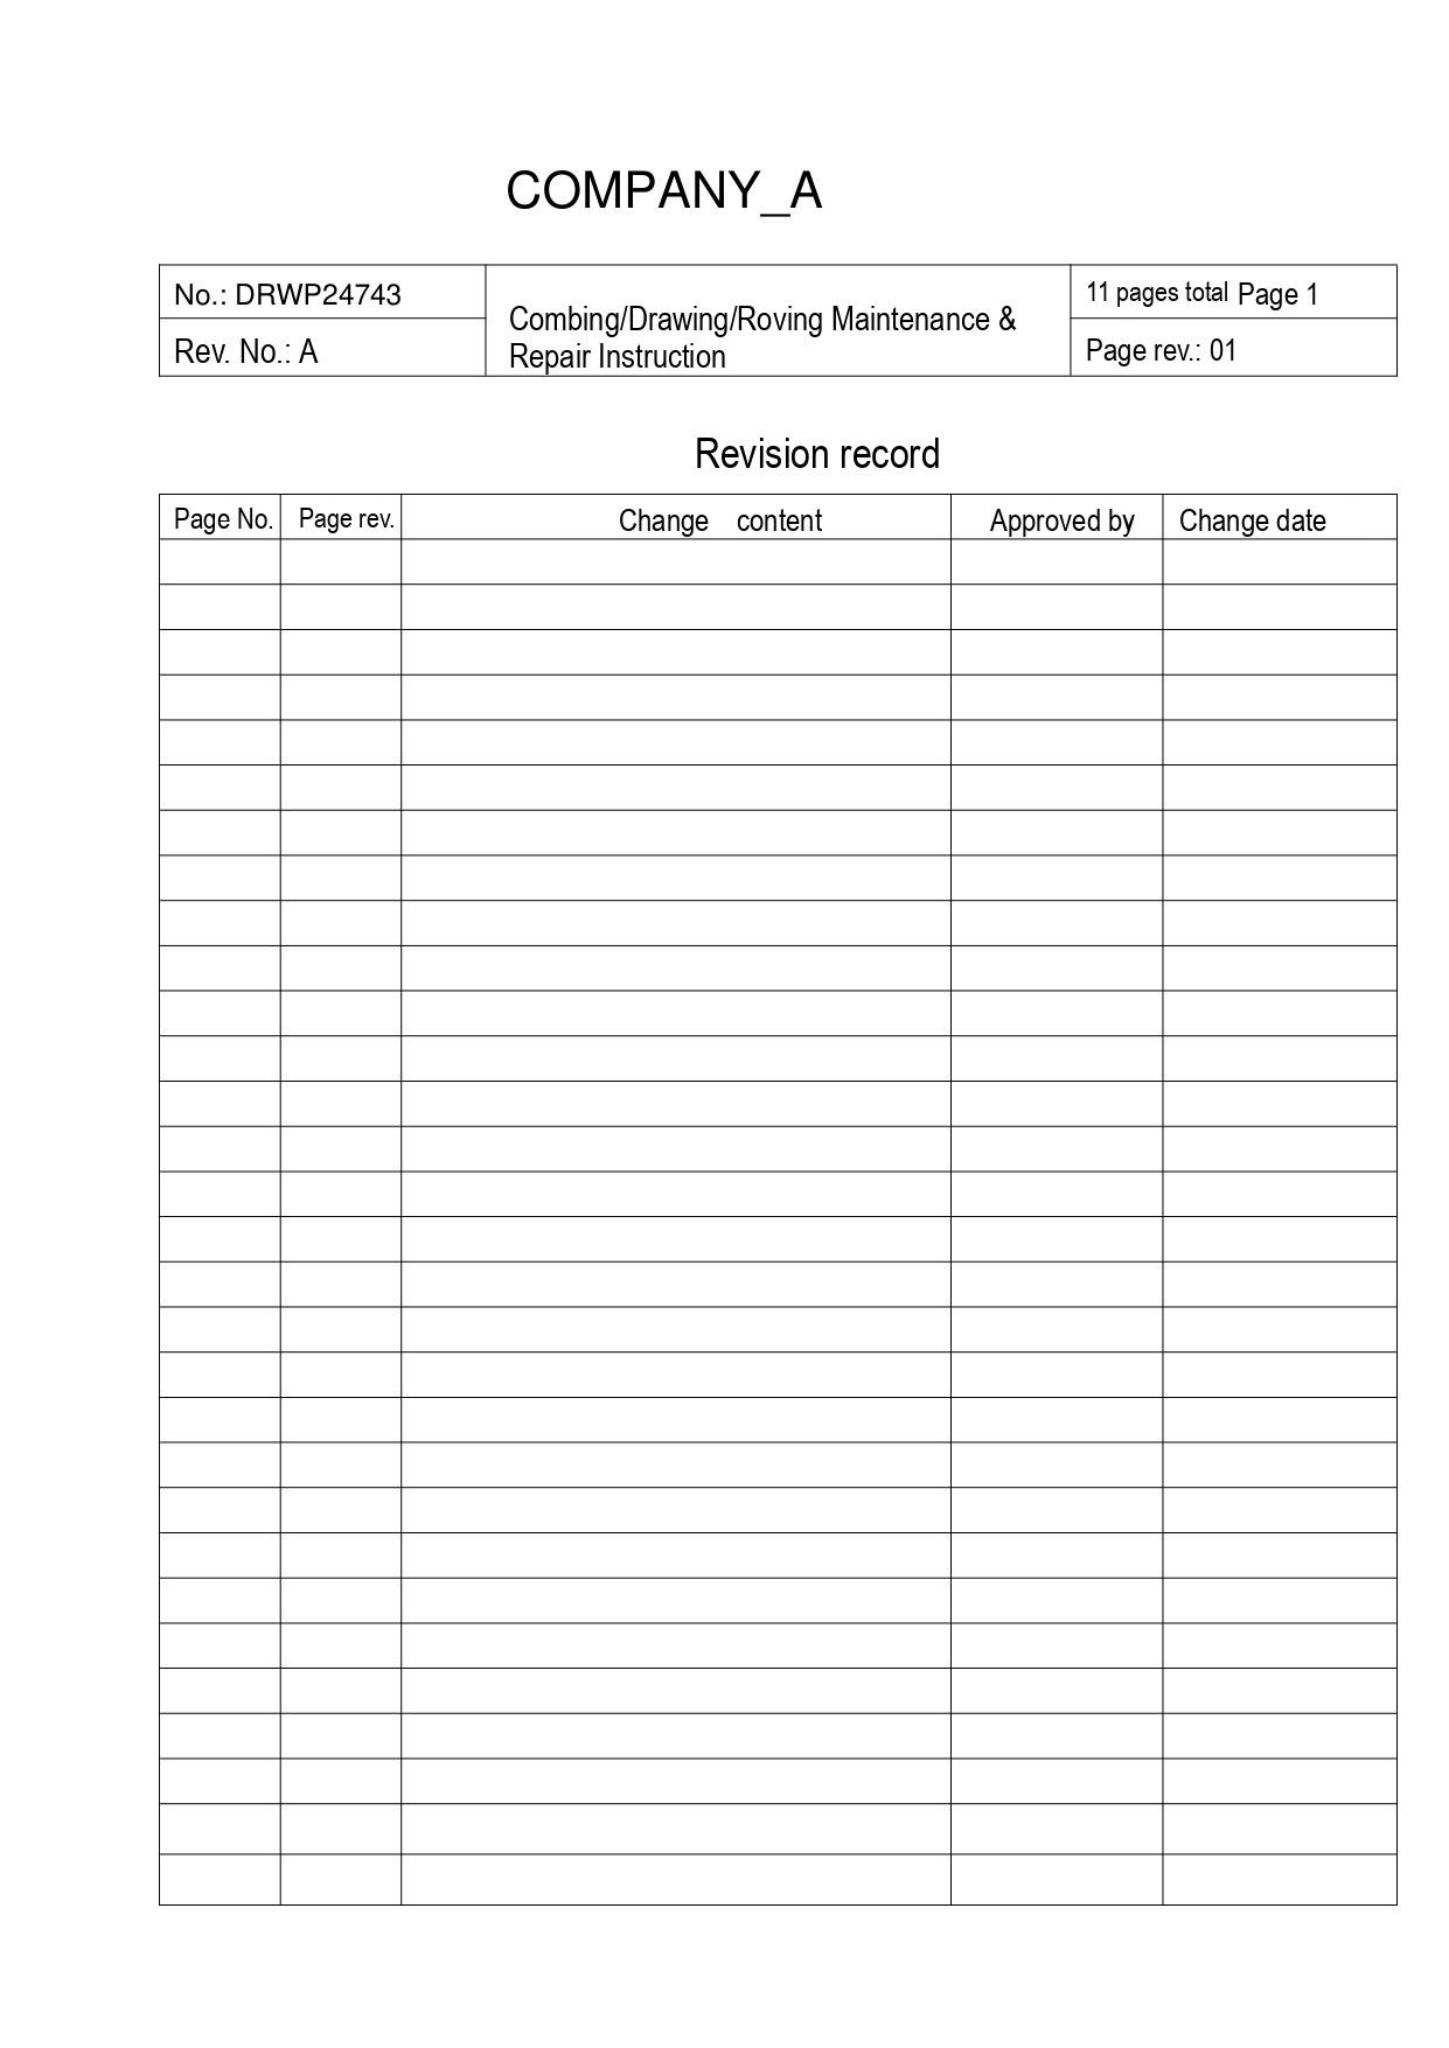COMPANY_A

| No.: DRWP24743 | Combing/Drawing/Roving Maintenance & Repair Instruction | 11 pages total Page 1 |
|---|---|---|
| Rev. No.: A | | Page rev.: 01 |

Revision record

| Page No. | Page rev. | Change content | Approved by | Change date |
|---|---|---|---|---|
| | | | | |
| | | | | |
| | | | | |
| | | | | |
| | | | | |
| | | | | |
| | | | | |
| | | | | |
| | | | | |
| | | | | |
| | | | | |
| | | | | |
| | | | | |
| | | | | |
| | | | | |
| | | | | |
| | | | | |
| | | | | |
| | | | | |
| | | | | |
| | | | | |
| | | | | |
| | | | | |
| | | | | |
| | | | | |
| | | | | |
| | | | | |
| | | | | |
| | | | | |
| | | | | |
| | | | | |
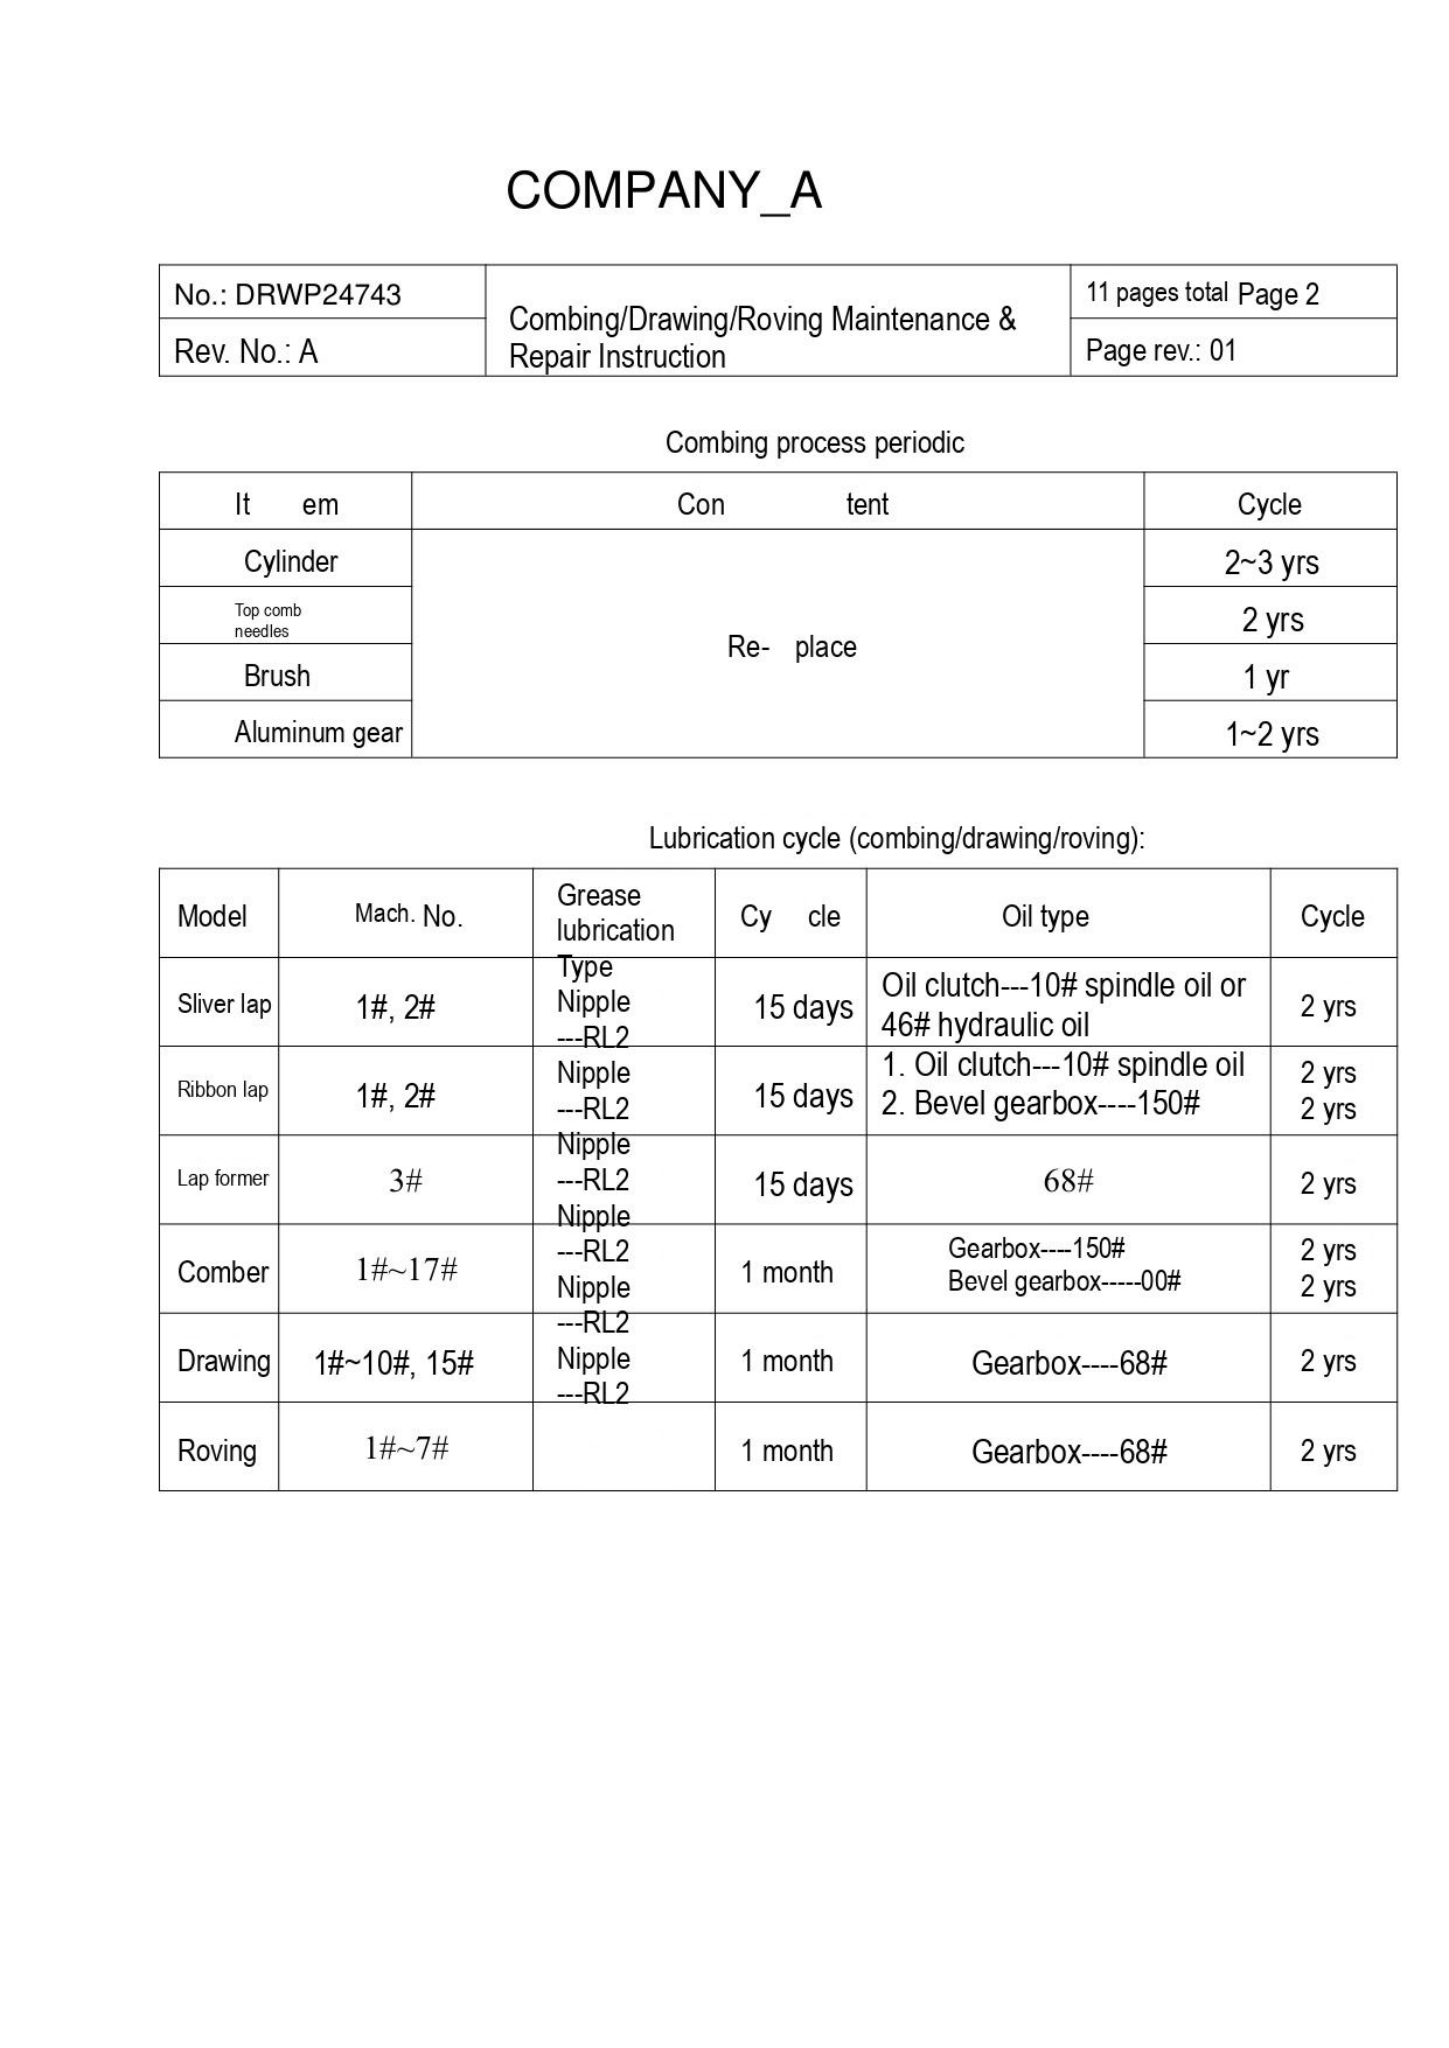COMPANY_A

| No.: DRWP24743 | Combing/Drawing/Roving Maintenance & Repair Instruction | 11 pages total Page 2 |
|---|---|---|
| Rev. No.: A | | Page rev.: 01 |

Combing process periodic

| It em | Con tent | Cycle |
|---|---|---|
| Cylinder | Re- place | 2~3 yrs |
| Top comb needles | | 2 yrs |
| Brush | | 1 yr |
| Aluminum gear | | 1~2 yrs |

Lubrication cycle (combing/drawing/roving):

| Model | Mach. No. | Grease lubrication Type | Cy cle | Oil type | Cycle |
|---|---|---|---|---|---|
| Sliver lap | 1#, 2# | Nipple ---RL2 | 15 days | Oil clutch---10# spindle oil or 46# hydraulic oil | 2 yrs |
| Ribbon lap | 1#, 2# | Nipple ---RL2 | 15 days | 1. Oil clutch---10# spindle oil<br>2. Bevel gearbox----150# | 2 yrs<br>2 yrs |
| Lap former | 3# | Nipple ---RL2 | 15 days | 68# | 2 yrs |
| Comber | 1#~17# | Nipple ---RL2<br>Nipple ---RL2 | 1 month | Gearbox----150#<br>Bevel gearbox-----00# | 2 yrs<br>2 yrs |
| Drawing | 1#~10#, 15# | Nipple ---RL2 | 1 month | Gearbox----68# | 2 yrs |
| Roving | 1#~7# | | 1 month | Gearbox----68# | 2 yrs |
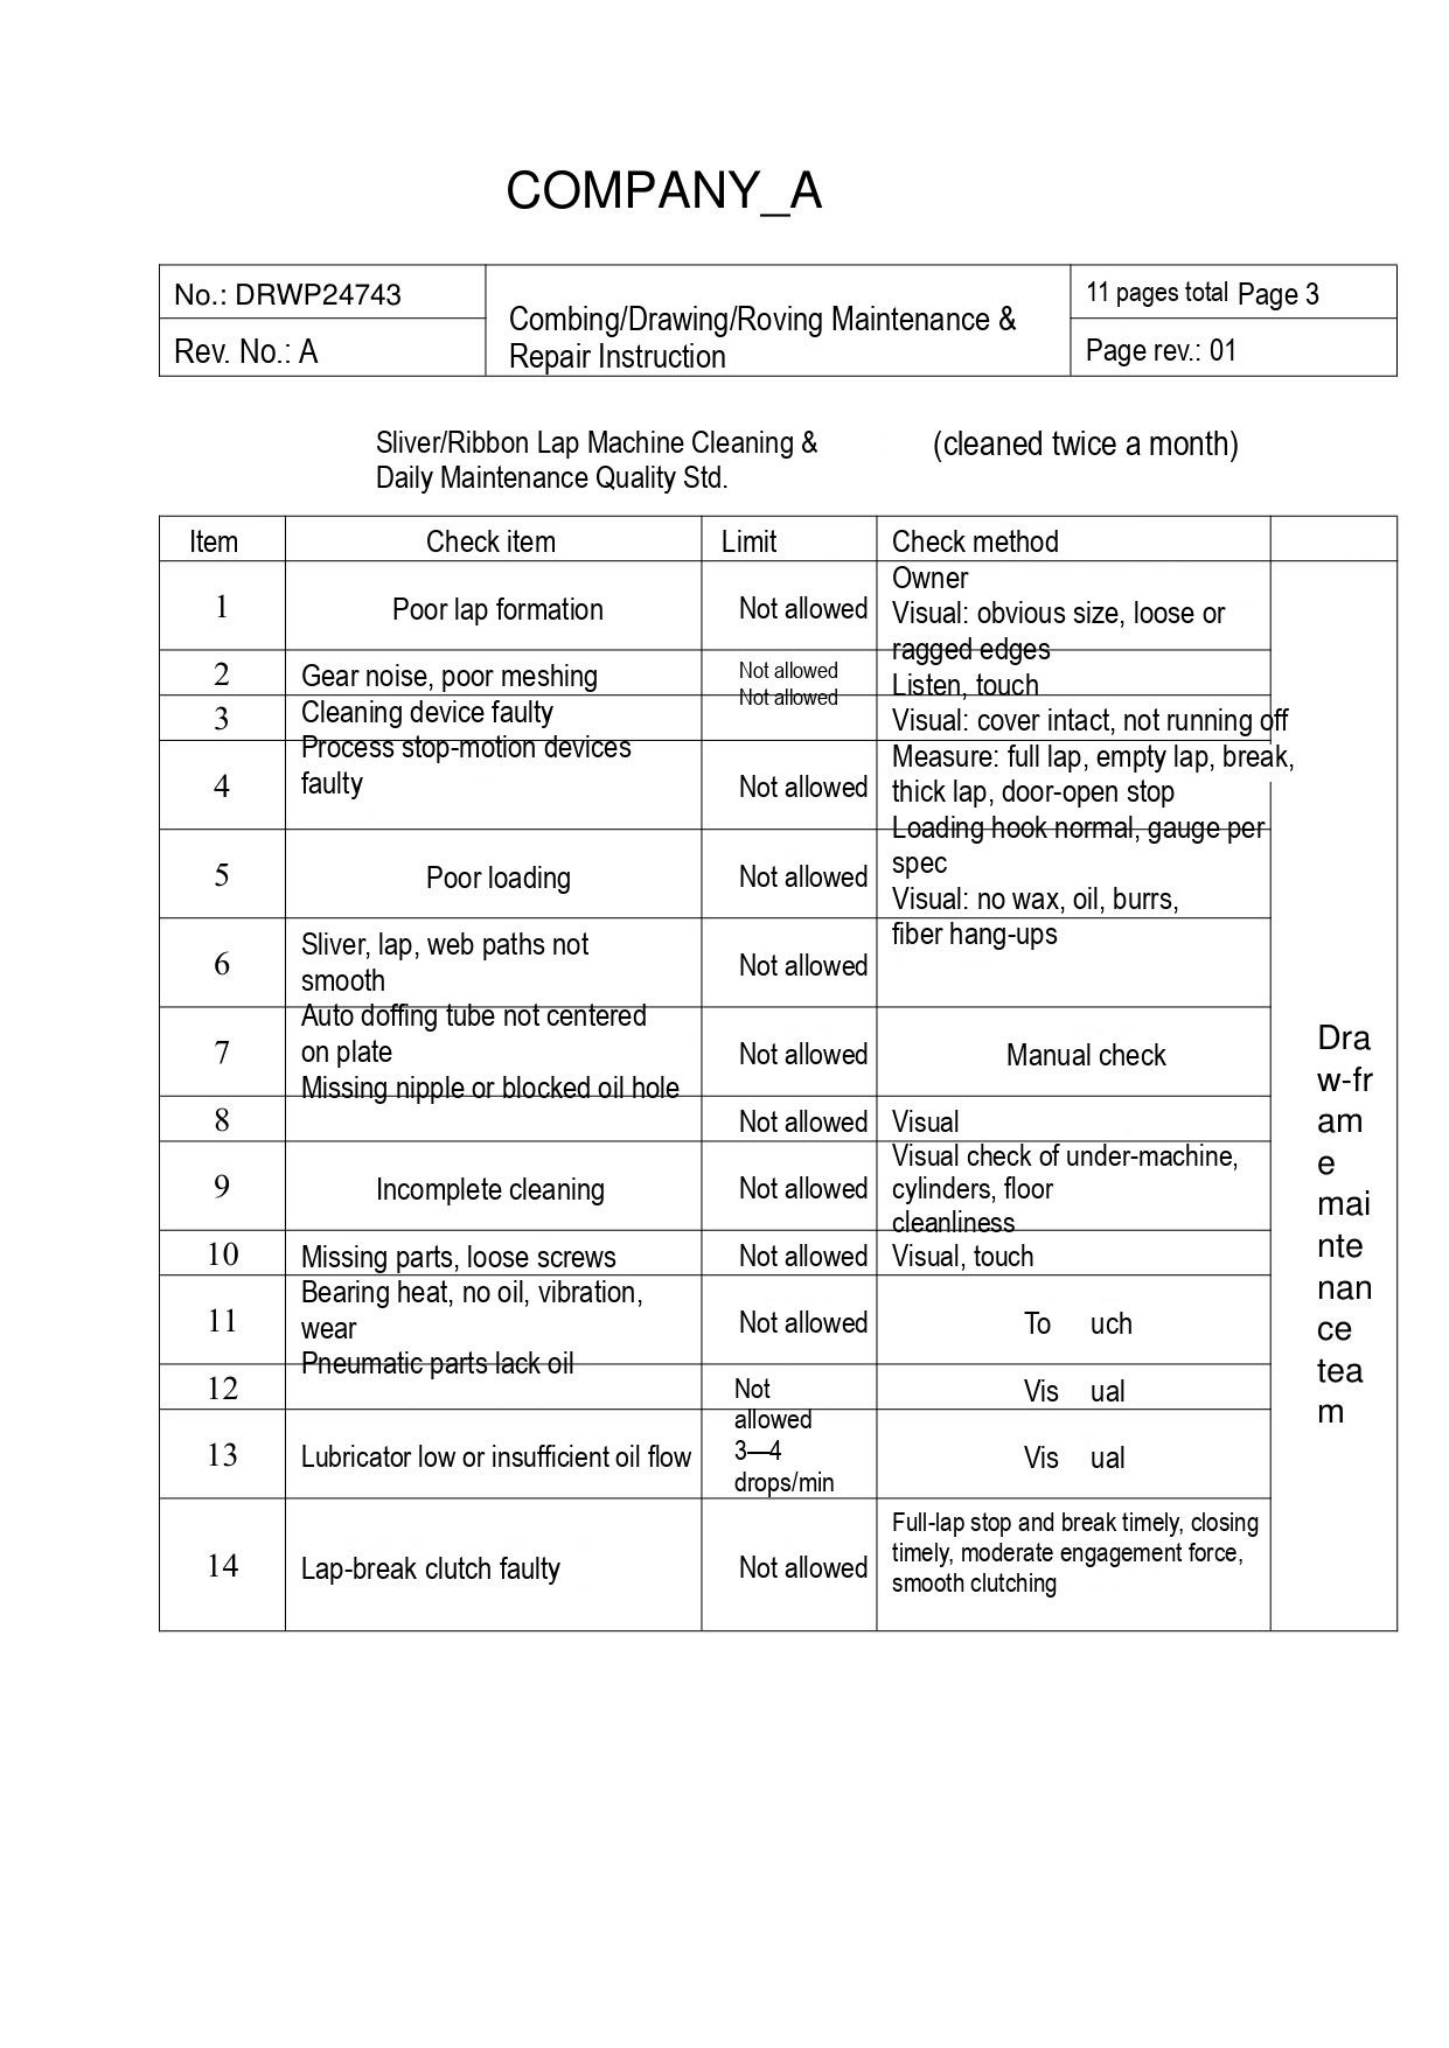# COMPANY_A

| No.: DRWP24743 | Combing/Drawing/Roving Maintenance & Repair Instruction | 11 pages total Page 3 |
|---|---|---|
| Rev. No.: A | | Page rev.: 01 |

Sliver/Ribbon Lap Machine Cleaning & Daily Maintenance Quality Std. (cleaned twice a month)

| Item | Check item | Limit | Check method | |
|---|---|---|---|---|
| 1 | Poor lap formation | Not allowed | Owner<br>Visual: obvious size, loose or ragged edges | Draw-frame maintenance team |
| 2 | Gear noise, poor meshing | Not allowed | Listen, touch | |
| 3 | Cleaning device faulty | Not allowed | Visual: cover intact, not running off | |
| 4 | Process stop-motion devices faulty | Not allowed | Measure: full lap, empty lap, break, thick lap, door-open stop | |
| 5 | Poor loading | Not allowed | Loading hook normal, gauge per spec | |
| 6 | Sliver, lap, web paths not smooth | Not allowed | Visual: no wax, oil, burrs, fiber hang-ups | |
| 7 | Auto doffing tube not centered on plate | Not allowed | Manual check | |
| 8 | Missing nipple or blocked oil hole | Not allowed | Visual | |
| 9 | Incomplete cleaning | Not allowed | Visual check of under-machine, cylinders, floor cleanliness | |
| 10 | Missing parts, loose screws | Not allowed | Visual, touch | |
| 11 | Bearing heat, no oil, vibration, wear | Not allowed | Touch | |
| 12 | Pneumatic parts lack oil | Not allowed | Visual | |
| 13 | Lubricator low or insufficient oil flow | 3—4 drops/min | Visual | |
| 14 | Lap-break clutch faulty | Not allowed | Full-lap stop and break timely, closing timely, moderate engagement force, smooth clutching | |
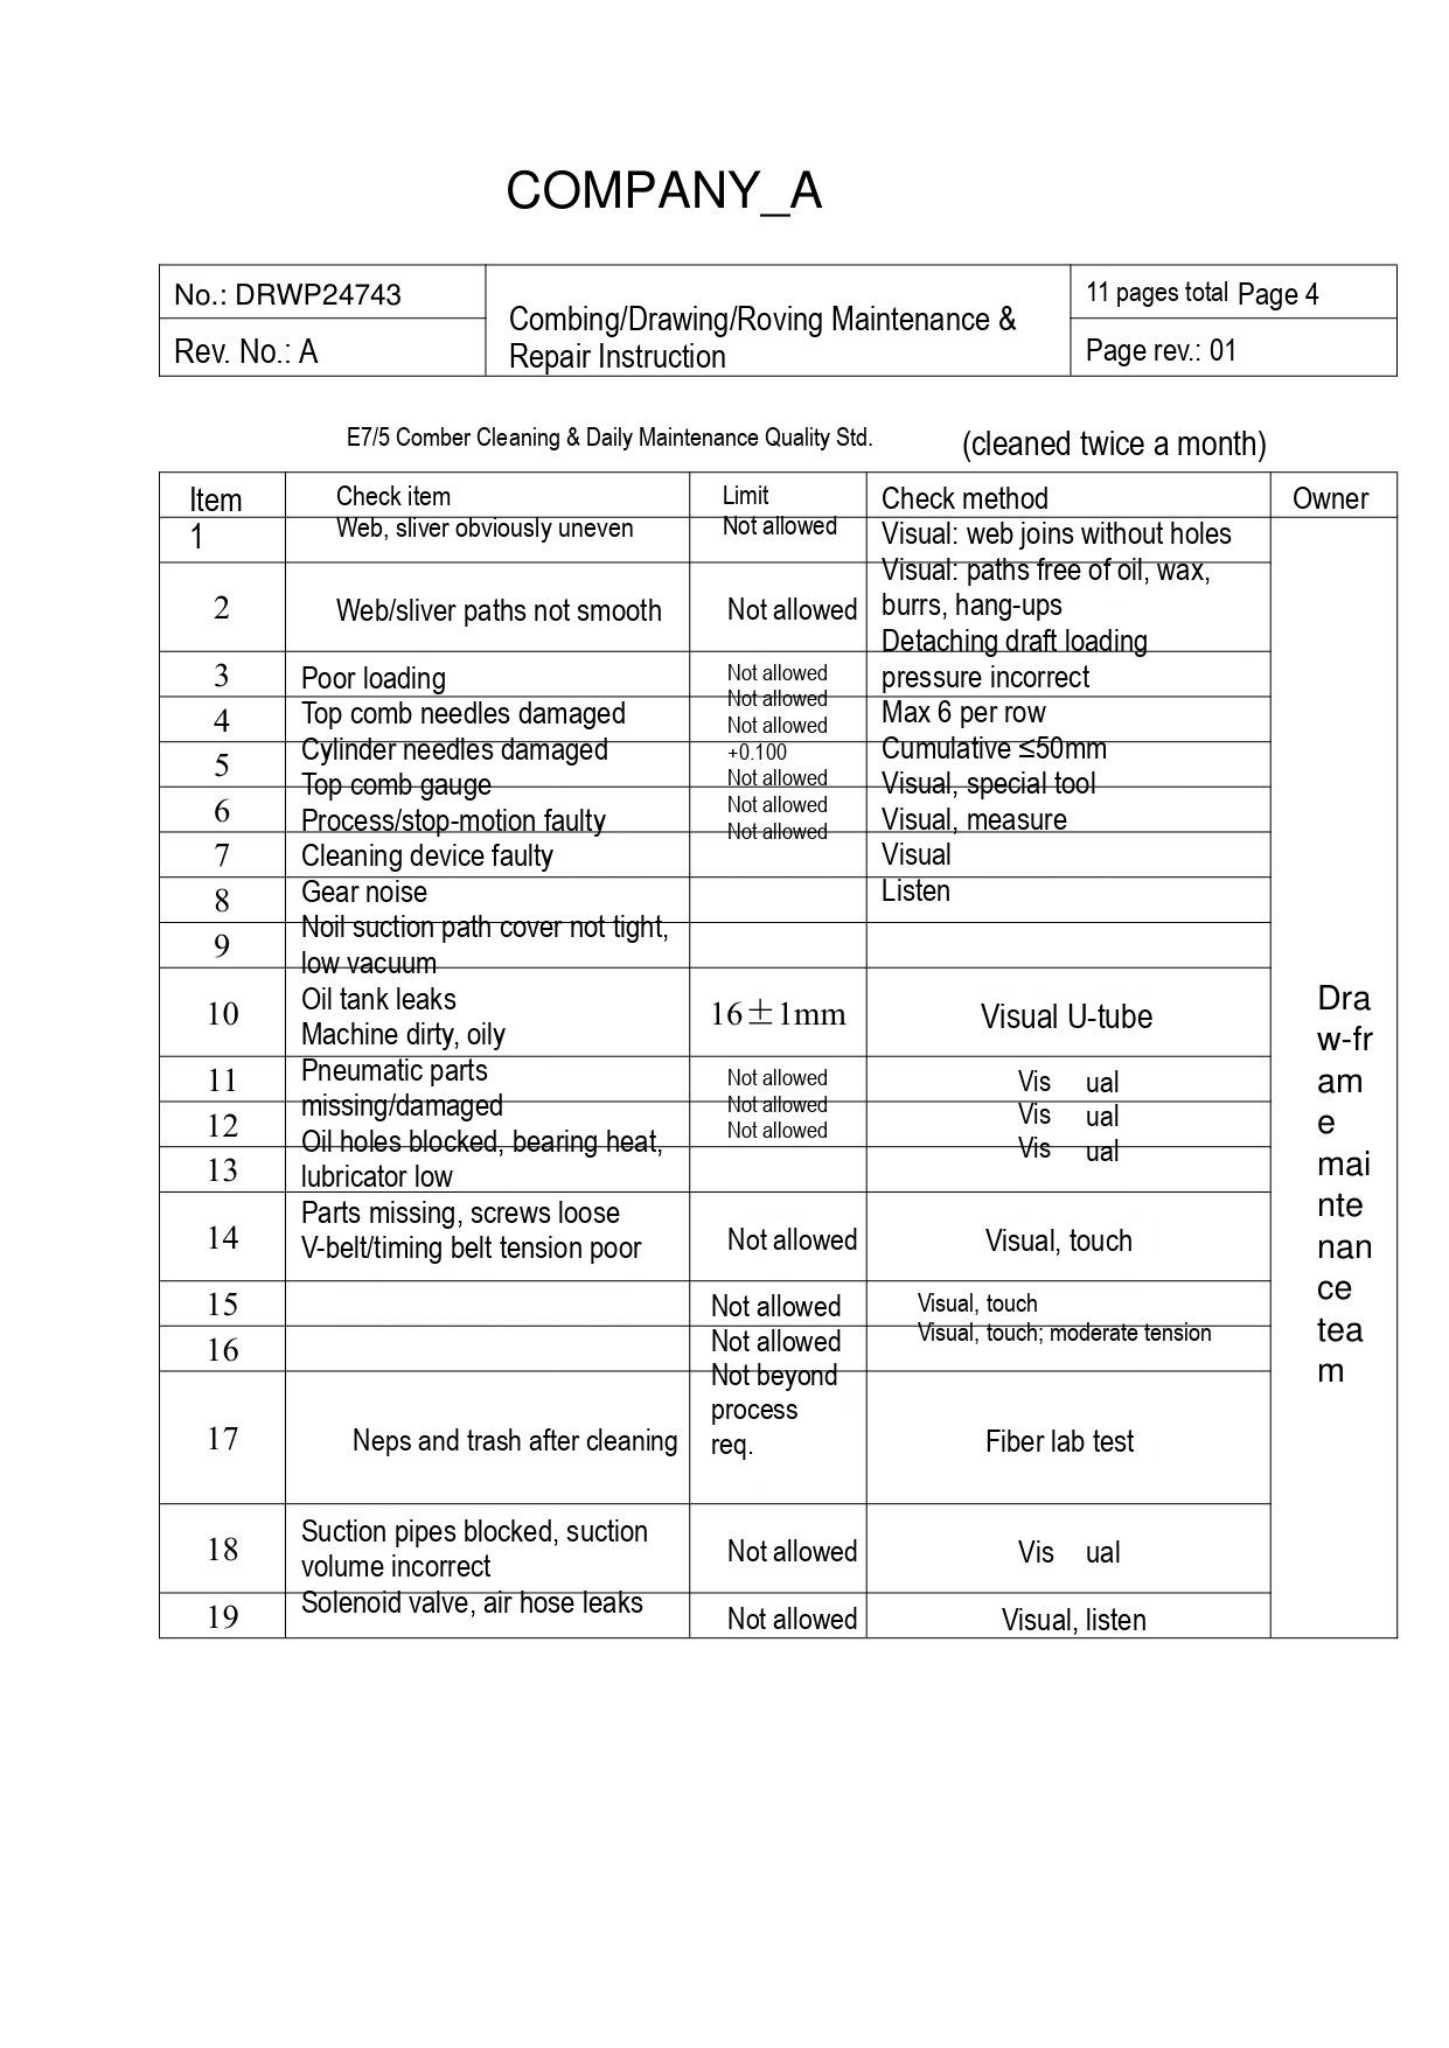# COMPANY_A

| No.: DRWP24743 | Combing/Drawing/Roving Maintenance & Repair Instruction | 11 pages total Page 4 |
|---|---|---|
| Rev. No.: A | | Page rev.: 01 |

E7/5 Comber Cleaning & Daily Maintenance Quality Std. (cleaned twice a month)

| Item | Check item | Limit | Check method | Owner |
|---|---|---|---|---|
| 1 | Web, sliver obviously uneven | Not allowed | Visual: web joins without holes | |
| 2 | Web/sliver paths not smooth | Not allowed | Visual: paths free of oil, wax, burrs, hang-ups | |
| 3 | Poor loading | Not allowed | Detaching draft loading pressure incorrect | |
| 4 | Top comb needles damaged | Not allowed<br>Not allowed | Max 6 per row | |
| 5 | Cylinder needles damaged | +0.100 | Cumulative ≤50mm | |
| 6 | Top comb gauge<br>Process/stop-motion faulty | Not allowed<br>Not allowed | Visual, special tool<br>Visual, measure | |
| 7 | Cleaning device faulty | Not allowed | Visual | |
| 8 | Gear noise | | Listen | |
| 9 | Noil suction path cover not tight, low vacuum | | | |
| 10 | Oil tank leaks<br>Machine dirty, oily | 16±1mm | Visual U-tube | Draw-frame maintenance team |
| 11 | Pneumatic parts missing/damaged | Not allowed | Visual | |
| 12 | Oil holes blocked, bearing heat, | Not allowed | Visual | |
| 13 | lubricator low | Not allowed | Visual | |
| 14 | Parts missing, screws loose<br>V-belt/timing belt tension poor | Not allowed | Visual, touch | |
| 15 | | Not allowed | Visual, touch | |
| 16 | | Not allowed | Visual, touch; moderate tension | |
| 17 | Neps and trash after cleaning | Not beyond process req. | Fiber lab test | |
| 18 | Suction pipes blocked, suction volume incorrect | Not allowed | Visual | |
| 19 | Solenoid valve, air hose leaks | Not allowed | Visual, listen | |
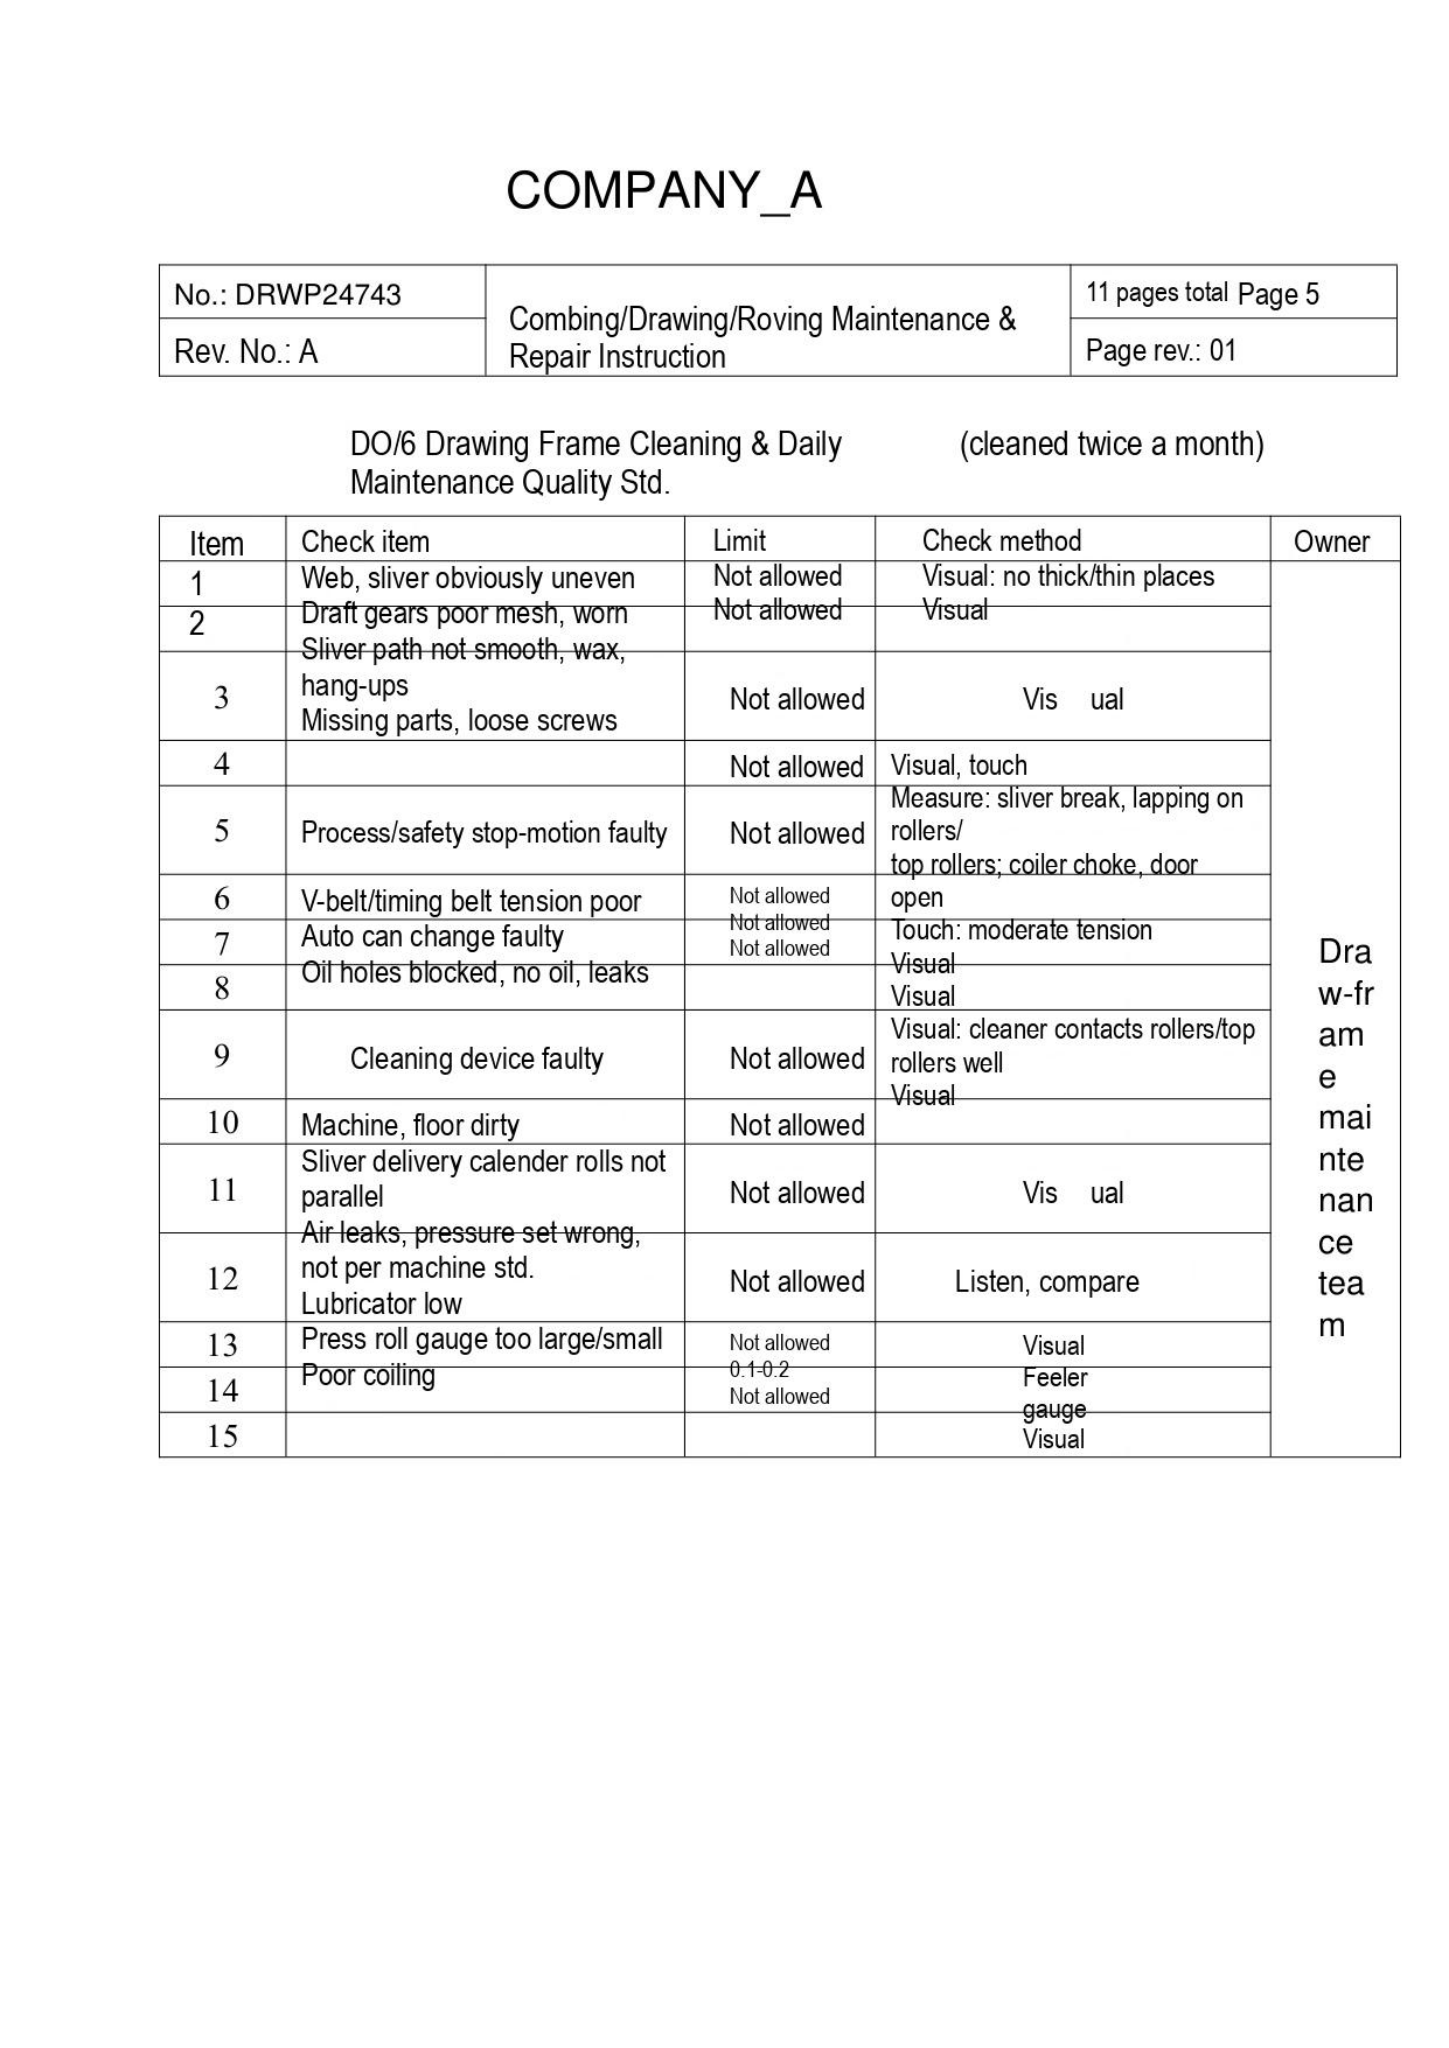# COMPANY_A

| No.: DRWP24743 | Combing/Drawing/Roving Maintenance & Repair Instruction | 11 pages total Page 5 |
|---|---|---|
| Rev. No.: A | | Page rev.: 01 |

DO/6 Drawing Frame Cleaning & Daily Maintenance Quality Std. (cleaned twice a month)

| Item | Check item | Limit | Check method | Owner |
|---|---|---|---|---|
| 1 | Web, sliver obviously uneven | Not allowed | Visual: no thick/thin places | Draw-frame maintenance team |
| 2 | Draft gears poor mesh, worn | Not allowed | Visual | |
| 3 | Sliver path not smooth, wax, hang-ups<br>Missing parts, loose screws | Not allowed | Vis ual | |
| 4 | | Not allowed | Visual, touch | |
| 5 | Process/safety stop-motion faulty | Not allowed | Measure: sliver break, lapping on rollers/<br>top rollers; coiler choke, door | |
| 6 | V-belt/timing belt tension poor | Not allowed<br>Not allowed<br>Not allowed | open | |
| 7 | Auto can change faulty | | Touch: moderate tension<br>Visual | |
| 8 | Oil holes blocked, no oil, leaks | | Visual | |
| 9 | Cleaning device faulty | Not allowed | Visual: cleaner contacts rollers/top rollers well<br>Visual | |
| 10 | Machine, floor dirty | Not allowed | | |
| 11 | Sliver delivery calender rolls not parallel | Not allowed | Vis ual | |
| 12 | Air leaks, pressure set wrong, not per machine std.<br>Lubricator low | Not allowed | Listen, compare | |
| 13 | Press roll gauge too large/small | Not allowed<br>0.1-0.2 | Visual | |
| 14 | Poor coiling | Not allowed | Feeler gauge | |
| 15 | | | Visual | |
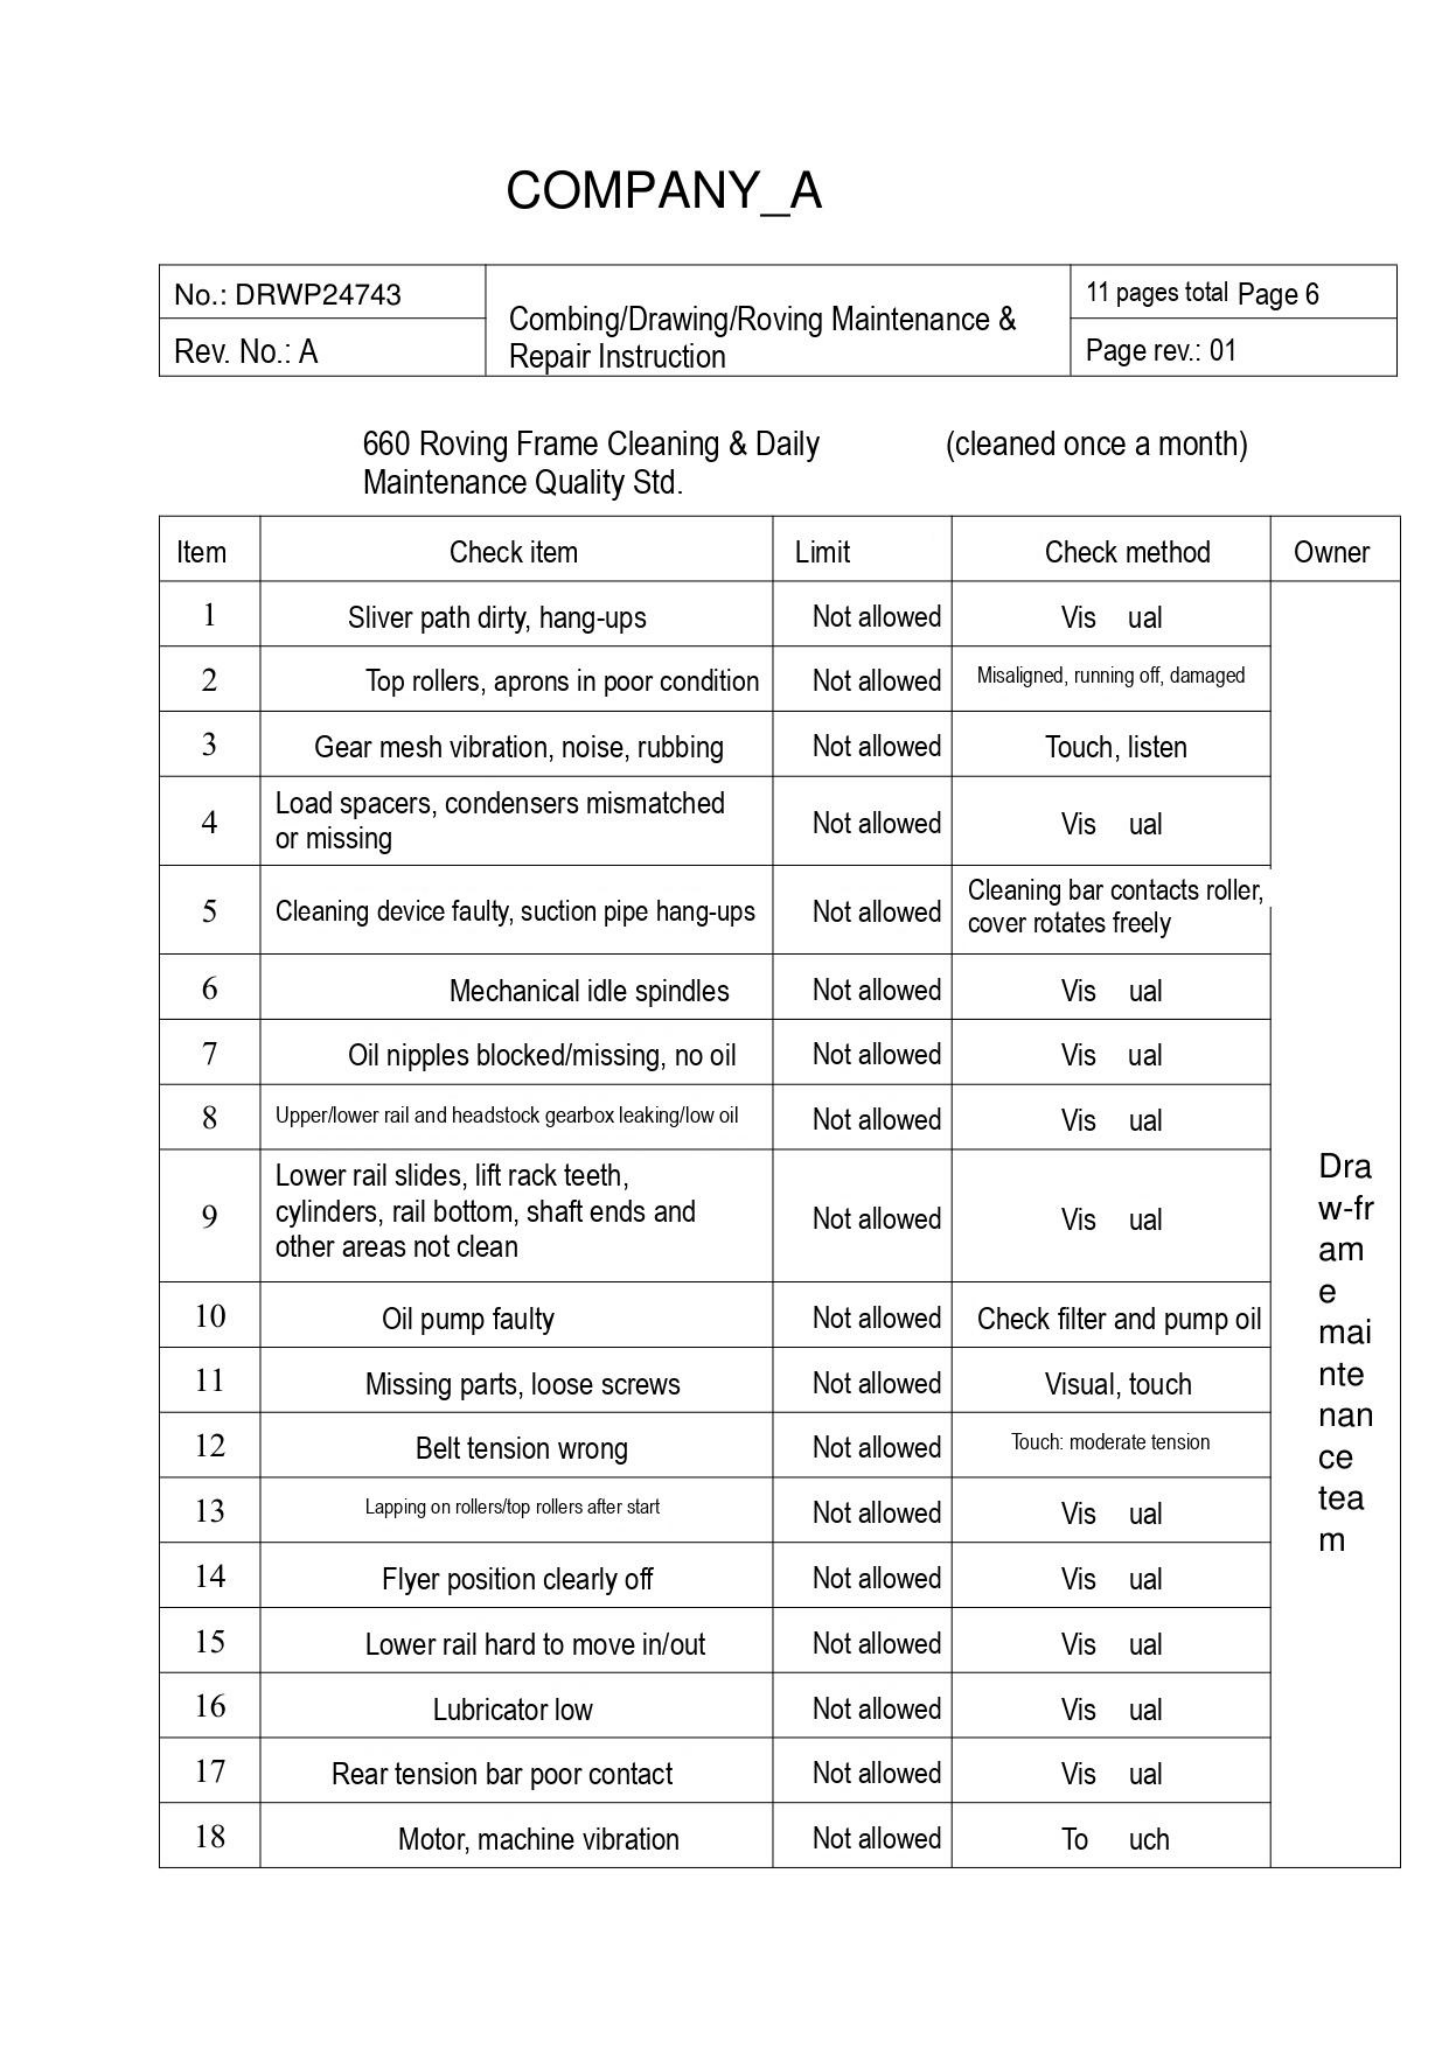COMPANY_A

| No.: DRWP24743 | Combing/Drawing/Roving Maintenance & Repair Instruction | 11 pages total Page 6 |
|---|---|---|
| Rev. No.: A | | Page rev.: 01 |

660 Roving Frame Cleaning & Daily Maintenance Quality Std. (cleaned once a month)

| Item | Check item | Limit | Check method | Owner |
|---|---|---|---|---|
| 1 | Sliver path dirty, hang-ups | Not allowed | Visual | Draw-frame maintenance team |
| 2 | Top rollers, aprons in poor condition | Not allowed | Misaligned, running off, damaged | |
| 3 | Gear mesh vibration, noise, rubbing | Not allowed | Touch, listen | |
| 4 | Load spacers, condensers mismatched or missing | Not allowed | Visual | |
| 5 | Cleaning device faulty, suction pipe hang-ups | Not allowed | Cleaning bar contacts roller, cover rotates freely | |
| 6 | Mechanical idle spindles | Not allowed | Visual | |
| 7 | Oil nipples blocked/missing, no oil | Not allowed | Visual | |
| 8 | Upper/lower rail and headstock gearbox leaking/low oil | Not allowed | Visual | |
| 9 | Lower rail slides, lift rack teeth, cylinders, rail bottom, shaft ends and other areas not clean | Not allowed | Visual | |
| 10 | Oil pump faulty | Not allowed | Check filter and pump oil | |
| 11 | Missing parts, loose screws | Not allowed | Visual, touch | |
| 12 | Belt tension wrong | Not allowed | Touch: moderate tension | |
| 13 | Lapping on rollers/top rollers after start | Not allowed | Visual | |
| 14 | Flyer position clearly off | Not allowed | Visual | |
| 15 | Lower rail hard to move in/out | Not allowed | Visual | |
| 16 | Lubricator low | Not allowed | Visual | |
| 17 | Rear tension bar poor contact | Not allowed | Visual | |
| 18 | Motor, machine vibration | Not allowed | Touch | |
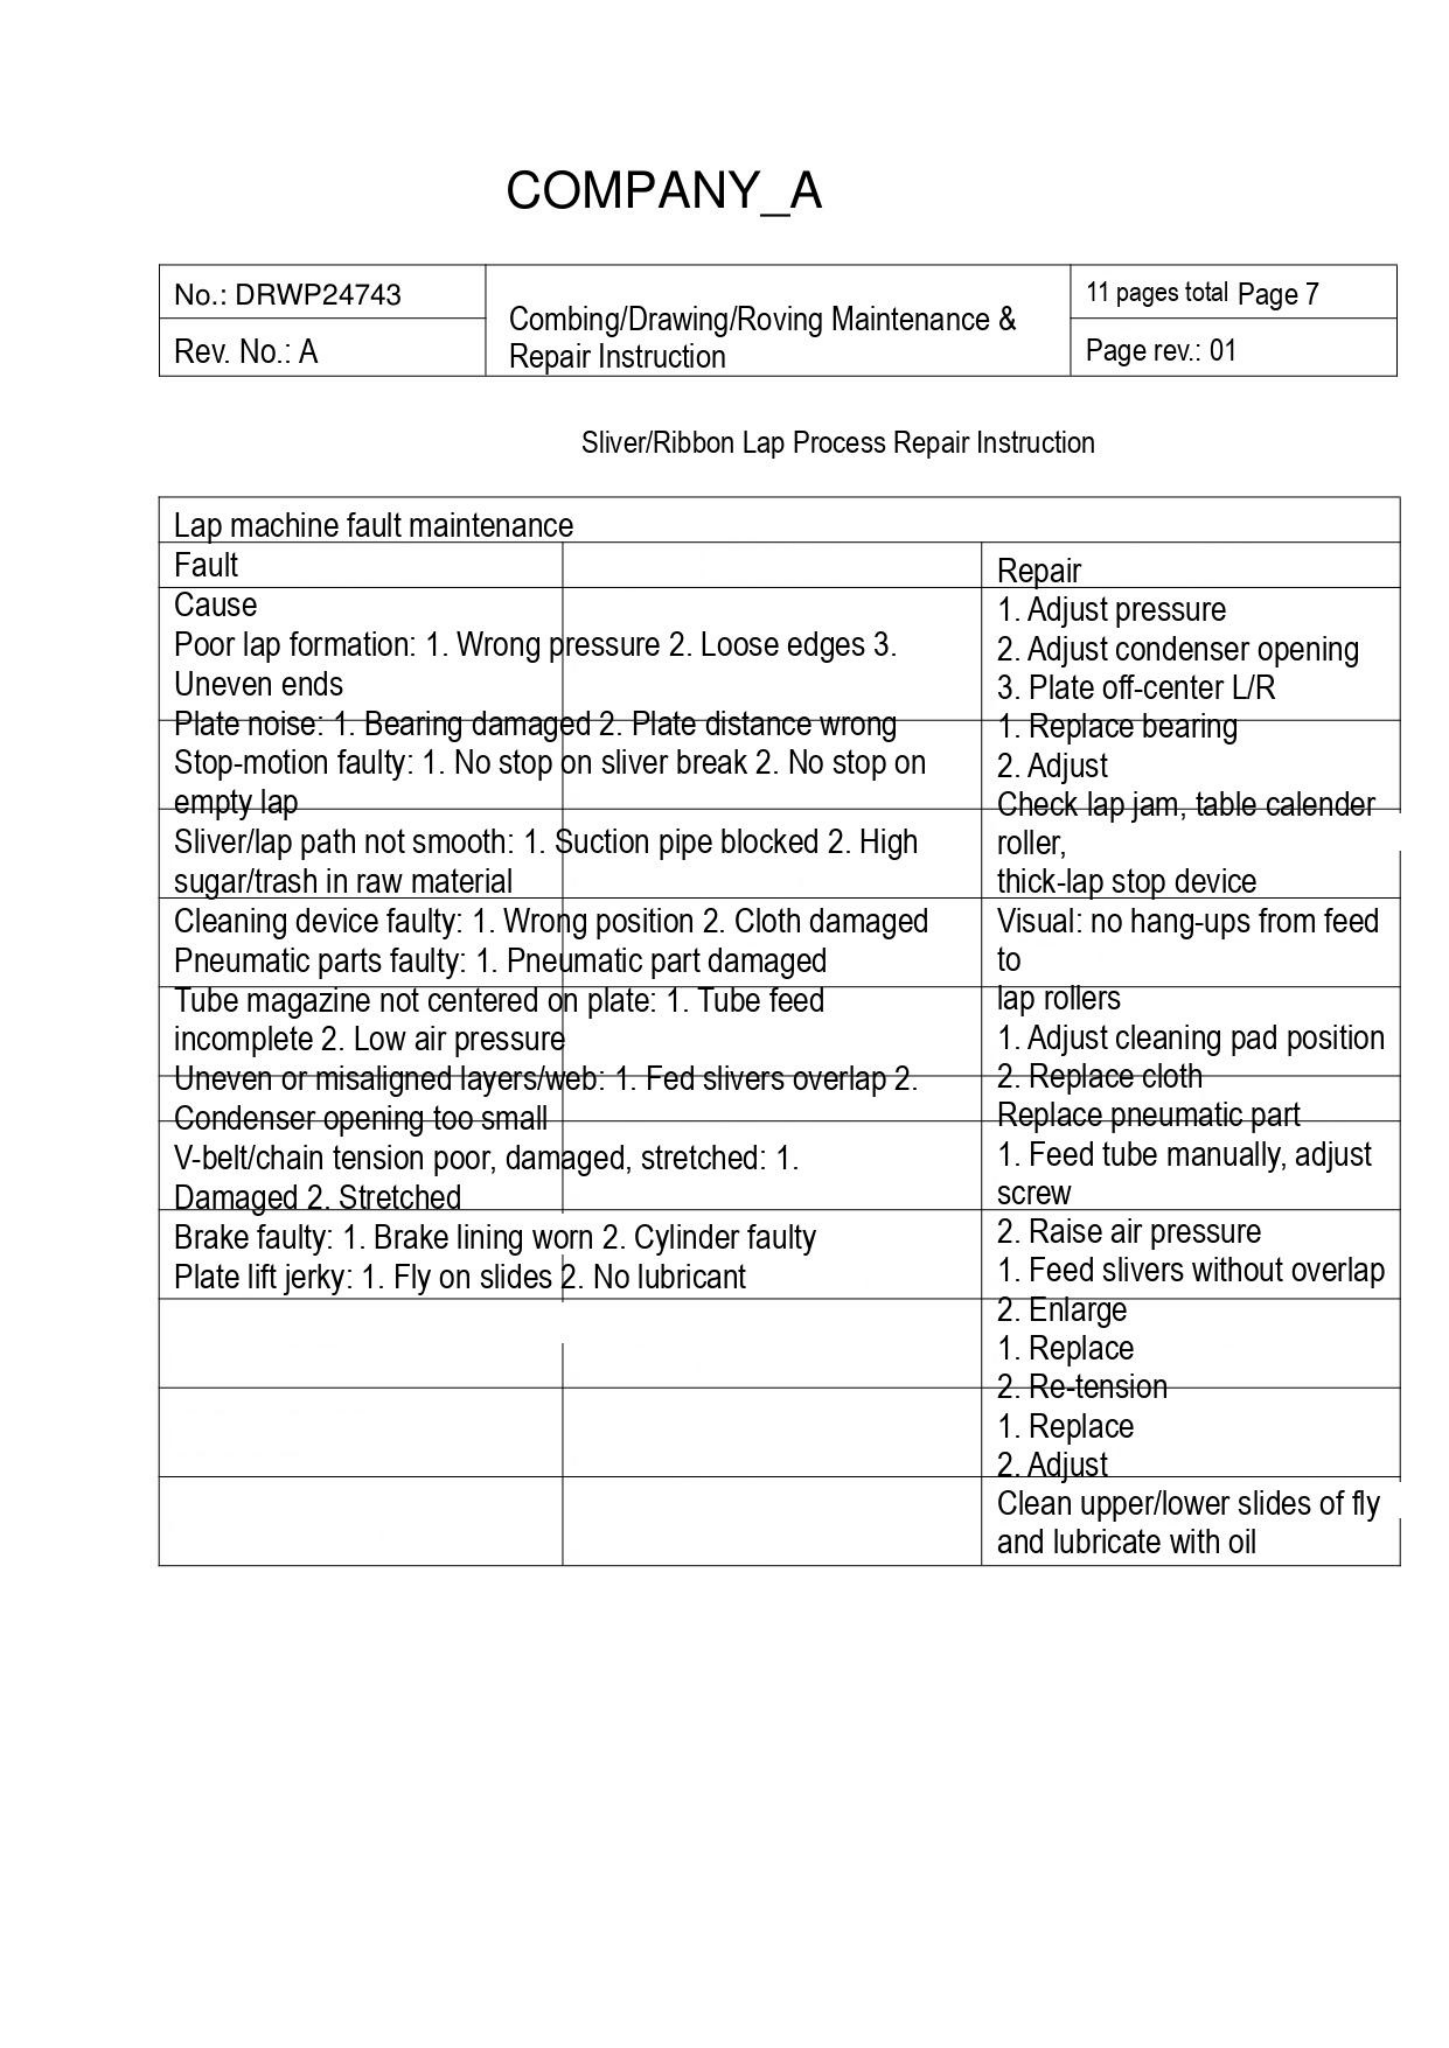# COMPANY_A

| No.: DRWP24743 | Combing/Drawing/Roving Maintenance & Repair Instruction | 11 pages total Page 7 |
|---|---|---|
| Rev. No.: A | | Page rev.: 01 |

Sliver/Ribbon Lap Process Repair Instruction

| Lap machine fault maintenance | | |
|---|---|---|
| Fault | | Repair |
| Cause<br>Poor lap formation: 1. Wrong pressure 2. Loose edges 3. Uneven ends | | 1. Adjust pressure<br>2. Adjust condenser opening<br>3. Plate off-center L/R |
| Plate noise: 1. Bearing damaged 2. Plate distance wrong<br>Stop-motion faulty: 1. No stop on sliver break 2. No stop on empty lap | | 1. Replace bearing<br>2. Adjust<br>Check lap jam, table calender |
| Sliver/lap path not smooth: 1. Suction pipe blocked 2. High sugar/trash in raw material | | roller,<br>thick-lap stop device |
| Cleaning device faulty: 1. Wrong position 2. Cloth damaged<br>Pneumatic parts faulty: 1. Pneumatic part damaged | | Visual: no hang-ups from feed to |
| Tube magazine not centered on plate: 1. Tube feed incomplete 2. Low air pressure | | lap rollers<br>1. Adjust cleaning pad position |
| Uneven or misaligned layers/web: 1. Fed slivers overlap 2. Condenser opening too small<br>V-belt/chain tension poor, damaged, stretched: 1. Damaged 2. Stretched | | 2. Replace cloth<br>Replace pneumatic part<br>1. Feed tube manually, adjust screw |
| Brake faulty: 1. Brake lining worn 2. Cylinder faulty<br>Plate lift jerky: 1. Fly on slides 2. No lubricant | | 2. Raise air pressure<br>1. Feed slivers without overlap |
| | | 2. Enlarge<br>1. Replace<br>2. Re-tension |
| | | 1. Replace<br>2. Adjust |
| | | Clean upper/lower slides of fly and lubricate with oil |